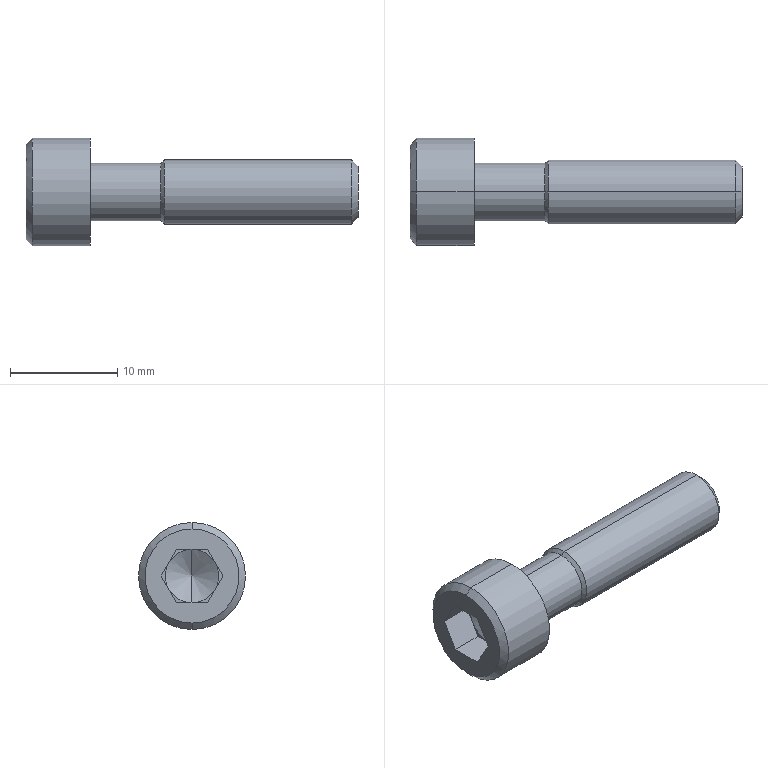Part | STEP file | 0245_Z_037_SCBS6-25_1 | 1 solid | 29 faces | box 31 x 10 x 10 mm | volume 1058 mm3 | plane 15 | cone 8 | cylinder 6 | commonest cylinder face diameters 5.386 x2 6 x2 10 x2